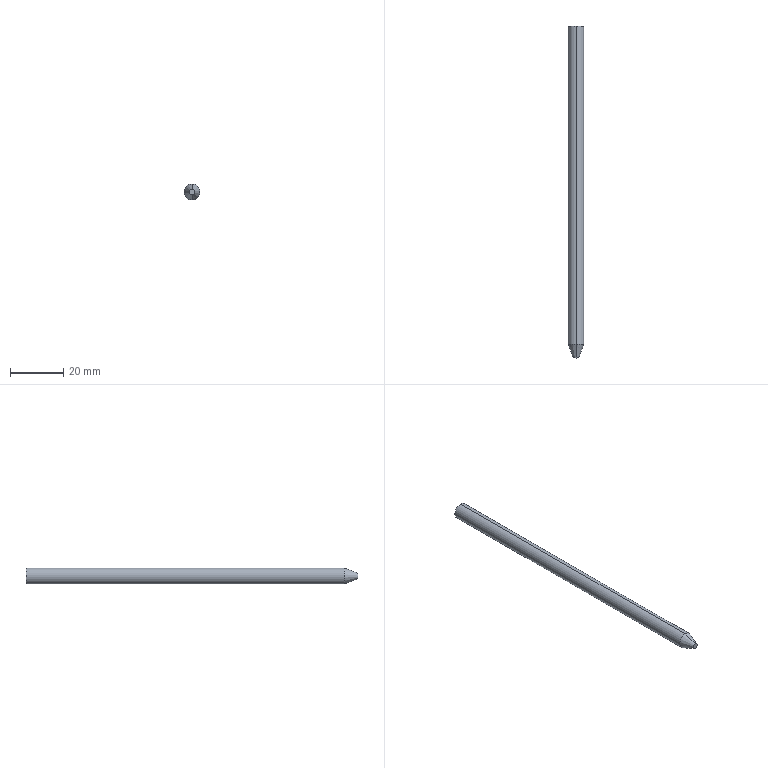Part | STEP file | Press rod | 1 solid | 6 faces | box 6 x 125 x 6 mm | volume 3458 mm3 | cylinder 2 | cone 2 | plane 2 | commonest cylinder face diameters 6 x2
STEP:
#1=CARTESIAN_POINT('',(0.,0.,0.));
#2=DIRECTION('',(0.,0.,1.));
#3=DIRECTION('',(1.,0.,0.));
#4=AXIS2_PLACEMENT_3D('',#1,#2,#3);
#5=CARTESIAN_POINT('',(22.704,-9.171,3.));
#6=VERTEX_POINT('',#5);
#7=CARTESIAN_POINT('',(22.704,-9.171,-3.));
#8=VERTEX_POINT('',#7);
#9=CARTESIAN_POINT('',(22.704,-9.171,0.));
#10=DIRECTION('',(0.,1.,0.));
#11=DIRECTION('',(0.,0.,1.));
#12=AXIS2_PLACEMENT_3D('',#9,#10,#11);
#13=CIRCLE('',#12,3.);
#14=CARTESIAN_POINT('',(22.704,-14.434,0.));
#15=DIRECTION('',(0.,1.,0.));
#16=DIRECTION('',(0.,0.,1.));
#17=AXIS2_PLACEMENT_3D('',#14,#15,#16);
#18=CYLINDRICAL_SURFACE('',#17,3.);
#19=CARTESIAN_POINT('',(0.,5.263));
#20=DIRECTION('',(1.,0.));
#21=VECTOR('',#20,1.);
#22=LINE('',#19,#21);
#23=(GEOMETRIC_REPRESENTATION_CONTEXT(2)PARAMETRIC_REPRESENTATION_CONTEXT()REPRESENTATION_CONTEXT('',''));
#24=DEFINITIONAL_REPRESENTATION('',(#22),#23);
#25=PCURVE('',#18,#24);
#26=CARTESIAN_POINT('',(22.704,-14.434,0.));
#27=DIRECTION('',(0.,1.,0.));
#28=DIRECTION('',(0.,0.,1.));
#29=AXIS2_PLACEMENT_3D('',#26,#27,#28);
#30=CONICAL_SURFACE('',#29,1.026,0.3588);
#31=CARTESIAN_POINT('',(0.,5.263));
#32=DIRECTION('',(1.,0.));
#33=VECTOR('',#32,1.);
#34=LINE('',#31,#33);
#35=(GEOMETRIC_REPRESENTATION_CONTEXT(2)PARAMETRIC_REPRESENTATION_CONTEXT()REPRESENTATION_CONTEXT('',''));
#36=DEFINITIONAL_REPRESENTATION('',(#34),#35);
#37=PCURVE('',#30,#36);
#38=SURFACE_CURVE('',#13,(#25,#37),.PCURVE_S1.);
#39=EDGE_CURVE('',#6,#8,#38,.T.);
#40=ORIENTED_EDGE('',*,*,#39,.T.);
#41=CARTESIAN_POINT('',(22.704,110.566,-3.));
#42=VERTEX_POINT('',#41);
#43=CARTESIAN_POINT('',(22.704,-14.434,-3.));
#44=DIRECTION('',(0.,1.,0.));
#45=VECTOR('',#44,1.);
#46=LINE('',#43,#45);
#47=CARTESIAN_POINT('',(3.142,0.));
#48=DIRECTION('',(0.,1.));
#49=VECTOR('',#48,1.);
#50=LINE('',#47,#49);
#51=(GEOMETRIC_REPRESENTATION_CONTEXT(2)PARAMETRIC_REPRESENTATION_CONTEXT()REPRESENTATION_CONTEXT('',''));
#52=DEFINITIONAL_REPRESENTATION('',(#50),#51);
#53=PCURVE('',#18,#52);
#54=CARTESIAN_POINT('',(22.704,-14.434,0.));
#55=DIRECTION('',(0.,1.,0.));
#56=DIRECTION('',(0.,0.,1.));
#57=AXIS2_PLACEMENT_3D('',#54,#55,#56);
#58=CYLINDRICAL_SURFACE('',#57,3.);
#59=CARTESIAN_POINT('',(3.142,0.));
#60=DIRECTION('',(0.,1.));
#61=VECTOR('',#60,1.);
#62=LINE('',#59,#61);
#63=(GEOMETRIC_REPRESENTATION_CONTEXT(2)PARAMETRIC_REPRESENTATION_CONTEXT()REPRESENTATION_CONTEXT('',''));
#64=DEFINITIONAL_REPRESENTATION('',(#62),#63);
#65=PCURVE('',#58,#64);
#66=SURFACE_CURVE('',#46,(#53,#65),.PCURVE_S1.);
#67=EDGE_CURVE('',#8,#42,#66,.T.);
#68=ORIENTED_EDGE('',*,*,#67,.T.);
#69=CARTESIAN_POINT('',(22.704,110.566,3.));
#70=VERTEX_POINT('',#69);
#71=CARTESIAN_POINT('',(22.704,110.566,0.));
#72=DIRECTION('',(0.,1.,0.));
#73=DIRECTION('',(0.,0.,1.));
#74=AXIS2_PLACEMENT_3D('',#71,#72,#73);
#75=CIRCLE('',#74,3.);
#76=CARTESIAN_POINT('',(0.,125.));
#77=DIRECTION('',(1.,0.));
#78=VECTOR('',#77,1.);
#79=LINE('',#76,#78);
#80=(GEOMETRIC_REPRESENTATION_CONTEXT(2)PARAMETRIC_REPRESENTATION_CONTEXT()REPRESENTATION_CONTEXT('',''));
#81=DEFINITIONAL_REPRESENTATION('',(#79),#80);
#82=PCURVE('',#18,#81);
#83=CARTESIAN_POINT('',(25.704,110.566,0.));
#84=DIRECTION('',(0.,-1.,0.));
#85=DIRECTION('',(0.,0.,-1.));
#86=AXIS2_PLACEMENT_3D('',#83,#84,#85);
#87=PLANE('',#86);
#88=CARTESIAN_POINT('',(-3.,-3.));
#89=CARTESIAN_POINT('',(-3.,2.196));
#90=CARTESIAN_POINT('',(1.5,-0.4019));
#91=CARTESIAN_POINT('',(6.,-3.));
#92=CARTESIAN_POINT('',(1.5,-5.598));
#93=CARTESIAN_POINT('',(-3.,-8.196));
#94=CARTESIAN_POINT('',(-3.,-3.));
#95=(BOUNDED_CURVE()B_SPLINE_CURVE(2,(#88,#89,#90,#91,#92,#93,#94),.UNSPECIFIED.,.T.,.F.)B_SPLINE_CURVE_WITH_KNOTS((1,2,2,2,2,1),(-2.094,0.,2.094,4.189,6.283,8.378),.UNSPECIFIED.)CURVE()GEOMETRIC_REPRESENTATION_ITEM()RATIONAL_B_SPLINE_CURVE((1.,0.5,1.,0.5,1.,0.5,1.))REPRESENTATION_ITEM(''));
#96=(GEOMETRIC_REPRESENTATION_CONTEXT(2)PARAMETRIC_REPRESENTATION_CONTEXT()REPRESENTATION_CONTEXT('',''));
#97=DEFINITIONAL_REPRESENTATION('',(#95),#96);
#98=PCURVE('',#87,#97);
#99=SURFACE_CURVE('',#75,(#82,#98),.PCURVE_S1.);
#100=EDGE_CURVE('',#70,#42,#99,.T.);
#101=ORIENTED_EDGE('',*,*,#100,.F.);
#102=CARTESIAN_POINT('',(22.704,-14.434,3.));
#103=DIRECTION('',(0.,1.,0.));
#104=VECTOR('',#103,1.);
#105=LINE('',#102,#104);
#106=CARTESIAN_POINT('',(0.,0.));
#107=DIRECTION('',(0.,1.));
#108=VECTOR('',#107,1.);
#109=LINE('',#106,#108);
#110=(GEOMETRIC_REPRESENTATION_CONTEXT(2)PARAMETRIC_REPRESENTATION_CONTEXT()REPRESENTATION_CONTEXT('',''));
#111=DEFINITIONAL_REPRESENTATION('',(#109),#110);
#112=PCURVE('',#18,#111);
#113=CARTESIAN_POINT('',(6.283,0.));
#114=DIRECTION('',(0.,1.));
#115=VECTOR('',#114,1.);
#116=LINE('',#113,#115);
#117=(GEOMETRIC_REPRESENTATION_CONTEXT(2)PARAMETRIC_REPRESENTATION_CONTEXT()REPRESENTATION_CONTEXT('',''));
#118=DEFINITIONAL_REPRESENTATION('',(#116),#117);
#119=PCURVE('',#58,#118);
#120=SURFACE_CURVE('',#105,(#112,#119),.PCURVE_S1.);
#121=EDGE_CURVE('',#6,#70,#120,.T.);
#122=ORIENTED_EDGE('',*,*,#121,.F.);
#123=EDGE_LOOP('',(#40,#68,#101,#122));
#124=FACE_BOUND('',#123,.T.);
#125=ADVANCED_FACE('',(#124),#18,.T.);
#126=CARTESIAN_POINT('',(22.704,-14.434,1.026));
#127=VERTEX_POINT('',#126);
#128=CARTESIAN_POINT('',(22.704,-14.434,-1.026));
#129=VERTEX_POINT('',#128);
#130=CARTESIAN_POINT('',(22.704,-14.434,0.));
#131=DIRECTION('',(0.,1.,0.));
#132=DIRECTION('',(0.,0.,1.));
#133=AXIS2_PLACEMENT_3D('',#130,#131,#132);
#134=CIRCLE('',#133,1.026);
#135=CARTESIAN_POINT('',(0.,0.));
#136=DIRECTION('',(1.,0.));
#137=VECTOR('',#136,1.);
#138=LINE('',#135,#137);
#139=(GEOMETRIC_REPRESENTATION_CONTEXT(2)PARAMETRIC_REPRESENTATION_CONTEXT()REPRESENTATION_CONTEXT('',''));
#140=DEFINITIONAL_REPRESENTATION('',(#138),#139);
#141=PCURVE('',#30,#140);
#142=CARTESIAN_POINT('',(22.704,-14.434,0.));
#143=DIRECTION('',(0.,1.,0.));
#144=DIRECTION('',(0.,0.,1.));
#145=AXIS2_PLACEMENT_3D('',#142,#143,#144);
#146=PLANE('',#145);
#147=CARTESIAN_POINT('',(0.,0.));
#148=DIRECTION('',(1.,0.));
#149=AXIS2_PLACEMENT_2D('',#147,#148);
#150=CIRCLE('',#149,1.026);
#151=(GEOMETRIC_REPRESENTATION_CONTEXT(2)PARAMETRIC_REPRESENTATION_CONTEXT()REPRESENTATION_CONTEXT('',''));
#152=DEFINITIONAL_REPRESENTATION('',(#150),#151);
#153=PCURVE('',#146,#152);
#154=SURFACE_CURVE('',#134,(#141,#153),.PCURVE_S1.);
#155=EDGE_CURVE('',#127,#129,#154,.T.);
#156=ORIENTED_EDGE('',*,*,#155,.T.);
#157=CARTESIAN_POINT('',(22.704,-14.434,-1.026));
#158=DIRECTION('',(0.,0.9363,-0.3512));
#159=VECTOR('',#158,1.);
#160=LINE('',#157,#159);
#161=CARTESIAN_POINT('',(3.142,0.));
#162=DIRECTION('',(0.,1.));
#163=VECTOR('',#162,1.);
#164=LINE('',#161,#163);
#165=(GEOMETRIC_REPRESENTATION_CONTEXT(2)PARAMETRIC_REPRESENTATION_CONTEXT()REPRESENTATION_CONTEXT('',''));
#166=DEFINITIONAL_REPRESENTATION('',(#164),#165);
#167=PCURVE('',#30,#166);
#168=CARTESIAN_POINT('',(22.704,-14.434,0.));
#169=DIRECTION('',(0.,1.,0.));
#170=DIRECTION('',(0.,0.,1.));
#171=AXIS2_PLACEMENT_3D('',#168,#169,#170);
#172=CONICAL_SURFACE('',#171,1.026,0.3588);
#173=CARTESIAN_POINT('',(3.142,0.));
#174=DIRECTION('',(0.,1.));
#175=VECTOR('',#174,1.);
#176=LINE('',#173,#175);
#177=(GEOMETRIC_REPRESENTATION_CONTEXT(2)PARAMETRIC_REPRESENTATION_CONTEXT()REPRESENTATION_CONTEXT('',''));
#178=DEFINITIONAL_REPRESENTATION('',(#176),#177);
#179=PCURVE('',#172,#178);
#180=SURFACE_CURVE('',#160,(#167,#179),.PCURVE_S1.);
#181=EDGE_CURVE('',#129,#8,#180,.T.);
#182=ORIENTED_EDGE('',*,*,#181,.T.);
#183=ORIENTED_EDGE('',*,*,#39,.F.);
#184=CARTESIAN_POINT('',(22.704,-14.434,1.026));
#185=DIRECTION('',(0.,0.9363,0.3512));
#186=VECTOR('',#185,1.);
#187=LINE('',#184,#186);
#188=CARTESIAN_POINT('',(0.,0.));
#189=DIRECTION('',(0.,1.));
#190=VECTOR('',#189,1.);
#191=LINE('',#188,#190);
#192=(GEOMETRIC_REPRESENTATION_CONTEXT(2)PARAMETRIC_REPRESENTATION_CONTEXT()REPRESENTATION_CONTEXT('',''));
#193=DEFINITIONAL_REPRESENTATION('',(#191),#192);
#194=PCURVE('',#30,#193);
#195=CARTESIAN_POINT('',(6.283,0.));
#196=DIRECTION('',(0.,1.));
#197=VECTOR('',#196,1.);
#198=LINE('',#195,#197);
#199=(GEOMETRIC_REPRESENTATION_CONTEXT(2)PARAMETRIC_REPRESENTATION_CONTEXT()REPRESENTATION_CONTEXT('',''));
#200=DEFINITIONAL_REPRESENTATION('',(#198),#199);
#201=PCURVE('',#172,#200);
#202=SURFACE_CURVE('',#187,(#194,#201),.PCURVE_S1.);
#203=EDGE_CURVE('',#127,#6,#202,.T.);
#204=ORIENTED_EDGE('',*,*,#203,.F.);
#205=EDGE_LOOP('',(#156,#182,#183,#204));
#206=FACE_BOUND('',#205,.T.);
#207=ADVANCED_FACE('',(#206),#30,.T.);
#208=ORIENTED_EDGE('',*,*,#100,.T.);
#209=CARTESIAN_POINT('',(22.704,110.566,0.));
#210=DIRECTION('',(0.,1.,0.));
#211=DIRECTION('',(0.,0.,1.));
#212=AXIS2_PLACEMENT_3D('',#209,#210,#211);
#213=CIRCLE('',#212,3.);
#214=CARTESIAN_POINT('',(-3.,-3.));
#215=CARTESIAN_POINT('',(-3.,2.196));
#216=CARTESIAN_POINT('',(1.5,-0.4019));
#217=CARTESIAN_POINT('',(6.,-3.));
#218=CARTESIAN_POINT('',(1.5,-5.598));
#219=CARTESIAN_POINT('',(-3.,-8.196));
#220=CARTESIAN_POINT('',(-3.,-3.));
#221=(BOUNDED_CURVE()B_SPLINE_CURVE(2,(#214,#215,#216,#217,#218,#219,#220),.UNSPECIFIED.,.T.,.F.)B_SPLINE_CURVE_WITH_KNOTS((1,2,2,2,2,1),(-2.094,0.,2.094,4.189,6.283,8.378),.UNSPECIFIED.)CURVE()GEOMETRIC_REPRESENTATION_ITEM()RATIONAL_B_SPLINE_CURVE((1.,0.5,1.,0.5,1.,0.5,1.))REPRESENTATION_ITEM(''));
#222=(GEOMETRIC_REPRESENTATION_CONTEXT(2)PARAMETRIC_REPRESENTATION_CONTEXT()REPRESENTATION_CONTEXT('',''));
#223=DEFINITIONAL_REPRESENTATION('',(#221),#222);
#224=PCURVE('',#87,#223);
#225=CARTESIAN_POINT('',(0.,125.));
#226=DIRECTION('',(1.,0.));
#227=VECTOR('',#226,1.);
#228=LINE('',#225,#227);
#229=(GEOMETRIC_REPRESENTATION_CONTEXT(2)PARAMETRIC_REPRESENTATION_CONTEXT()REPRESENTATION_CONTEXT('',''));
#230=DEFINITIONAL_REPRESENTATION('',(#228),#229);
#231=PCURVE('',#58,#230);
#232=SURFACE_CURVE('',#213,(#224,#231),.PCURVE_S1.);
#233=EDGE_CURVE('',#42,#70,#232,.T.);
#234=ORIENTED_EDGE('',*,*,#233,.T.);
#235=EDGE_LOOP('',(#208,#234));
#236=FACE_BOUND('',#235,.T.);
#237=ADVANCED_FACE('',(#236),#87,.F.);
#238=ORIENTED_EDGE('',*,*,#155,.F.);
#239=CARTESIAN_POINT('',(22.704,-14.434,0.));
#240=DIRECTION('',(0.,1.,0.));
#241=DIRECTION('',(0.,0.,1.));
#242=AXIS2_PLACEMENT_3D('',#239,#240,#241);
#243=CIRCLE('',#242,1.026);
#244=CARTESIAN_POINT('',(0.,0.));
#245=DIRECTION('',(1.,0.));
#246=AXIS2_PLACEMENT_2D('',#244,#245);
#247=CIRCLE('',#246,1.026);
#248=(GEOMETRIC_REPRESENTATION_CONTEXT(2)PARAMETRIC_REPRESENTATION_CONTEXT()REPRESENTATION_CONTEXT('',''));
#249=DEFINITIONAL_REPRESENTATION('',(#247),#248);
#250=PCURVE('',#146,#249);
#251=CARTESIAN_POINT('',(0.,0.));
#252=DIRECTION('',(1.,0.));
#253=VECTOR('',#252,1.);
#254=LINE('',#251,#253);
#255=(GEOMETRIC_REPRESENTATION_CONTEXT(2)PARAMETRIC_REPRESENTATION_CONTEXT()REPRESENTATION_CONTEXT('',''));
#256=DEFINITIONAL_REPRESENTATION('',(#254),#255);
#257=PCURVE('',#172,#256);
#258=SURFACE_CURVE('',#243,(#250,#257),.PCURVE_S1.);
#259=EDGE_CURVE('',#129,#127,#258,.T.);
#260=ORIENTED_EDGE('',*,*,#259,.F.);
#261=EDGE_LOOP('',(#238,#260));
#262=FACE_BOUND('',#261,.T.);
#263=ADVANCED_FACE('',(#262),#146,.F.);
#264=ORIENTED_EDGE('',*,*,#181,.F.);
#265=ORIENTED_EDGE('',*,*,#259,.T.);
#266=ORIENTED_EDGE('',*,*,#203,.T.);
#267=CARTESIAN_POINT('',(22.704,-9.171,0.));
#268=DIRECTION('',(0.,1.,0.));
#269=DIRECTION('',(0.,0.,1.));
#270=AXIS2_PLACEMENT_3D('',#267,#268,#269);
#271=CIRCLE('',#270,3.);
#272=CARTESIAN_POINT('',(0.,5.263));
#273=DIRECTION('',(1.,0.));
#274=VECTOR('',#273,1.);
#275=LINE('',#272,#274);
#276=(GEOMETRIC_REPRESENTATION_CONTEXT(2)PARAMETRIC_REPRESENTATION_CONTEXT()REPRESENTATION_CONTEXT('',''));
#277=DEFINITIONAL_REPRESENTATION('',(#275),#276);
#278=PCURVE('',#172,#277);
#279=CARTESIAN_POINT('',(0.,5.263));
#280=DIRECTION('',(1.,0.));
#281=VECTOR('',#280,1.);
#282=LINE('',#279,#281);
#283=(GEOMETRIC_REPRESENTATION_CONTEXT(2)PARAMETRIC_REPRESENTATION_CONTEXT()REPRESENTATION_CONTEXT('',''));
#284=DEFINITIONAL_REPRESENTATION('',(#282),#283);
#285=PCURVE('',#58,#284);
#286=SURFACE_CURVE('',#271,(#278,#285),.PCURVE_S1.);
#287=EDGE_CURVE('',#8,#6,#286,.T.);
#288=ORIENTED_EDGE('',*,*,#287,.F.);
#289=EDGE_LOOP('',(#264,#265,#266,#288));
#290=FACE_BOUND('',#289,.T.);
#291=ADVANCED_FACE('',(#290),#172,.T.);
#292=ORIENTED_EDGE('',*,*,#67,.F.);
#293=ORIENTED_EDGE('',*,*,#287,.T.);
#294=ORIENTED_EDGE('',*,*,#121,.T.);
#295=ORIENTED_EDGE('',*,*,#233,.F.);
#296=EDGE_LOOP('',(#292,#293,#294,#295));
#297=FACE_BOUND('',#296,.T.);
#298=ADVANCED_FACE('',(#297),#58,.T.);
#299=CLOSED_SHELL('',(#125,#207,#237,#263,#291,#298));
#300=MANIFOLD_SOLID_BREP('',#299);
#301=(LENGTH_UNIT()NAMED_UNIT(*)SI_UNIT(.MILLI.,.METRE.));
#302=UNCERTAINTY_MEASURE_WITH_UNIT(LENGTH_MEASURE(0.0000001),#301,'','');
#303=(NAMED_UNIT(*)PLANE_ANGLE_UNIT()SI_UNIT($,.RADIAN.));
#304=(NAMED_UNIT(*)SI_UNIT($,.STERADIAN.)SOLID_ANGLE_UNIT());
#305=(GEOMETRIC_REPRESENTATION_CONTEXT(3)GLOBAL_UNCERTAINTY_ASSIGNED_CONTEXT((#302))GLOBAL_UNIT_ASSIGNED_CONTEXT((#301,#303,#304))REPRESENTATION_CONTEXT('',''));
#306=ADVANCED_BREP_SHAPE_REPRESENTATION('',(#4,#300),#305);